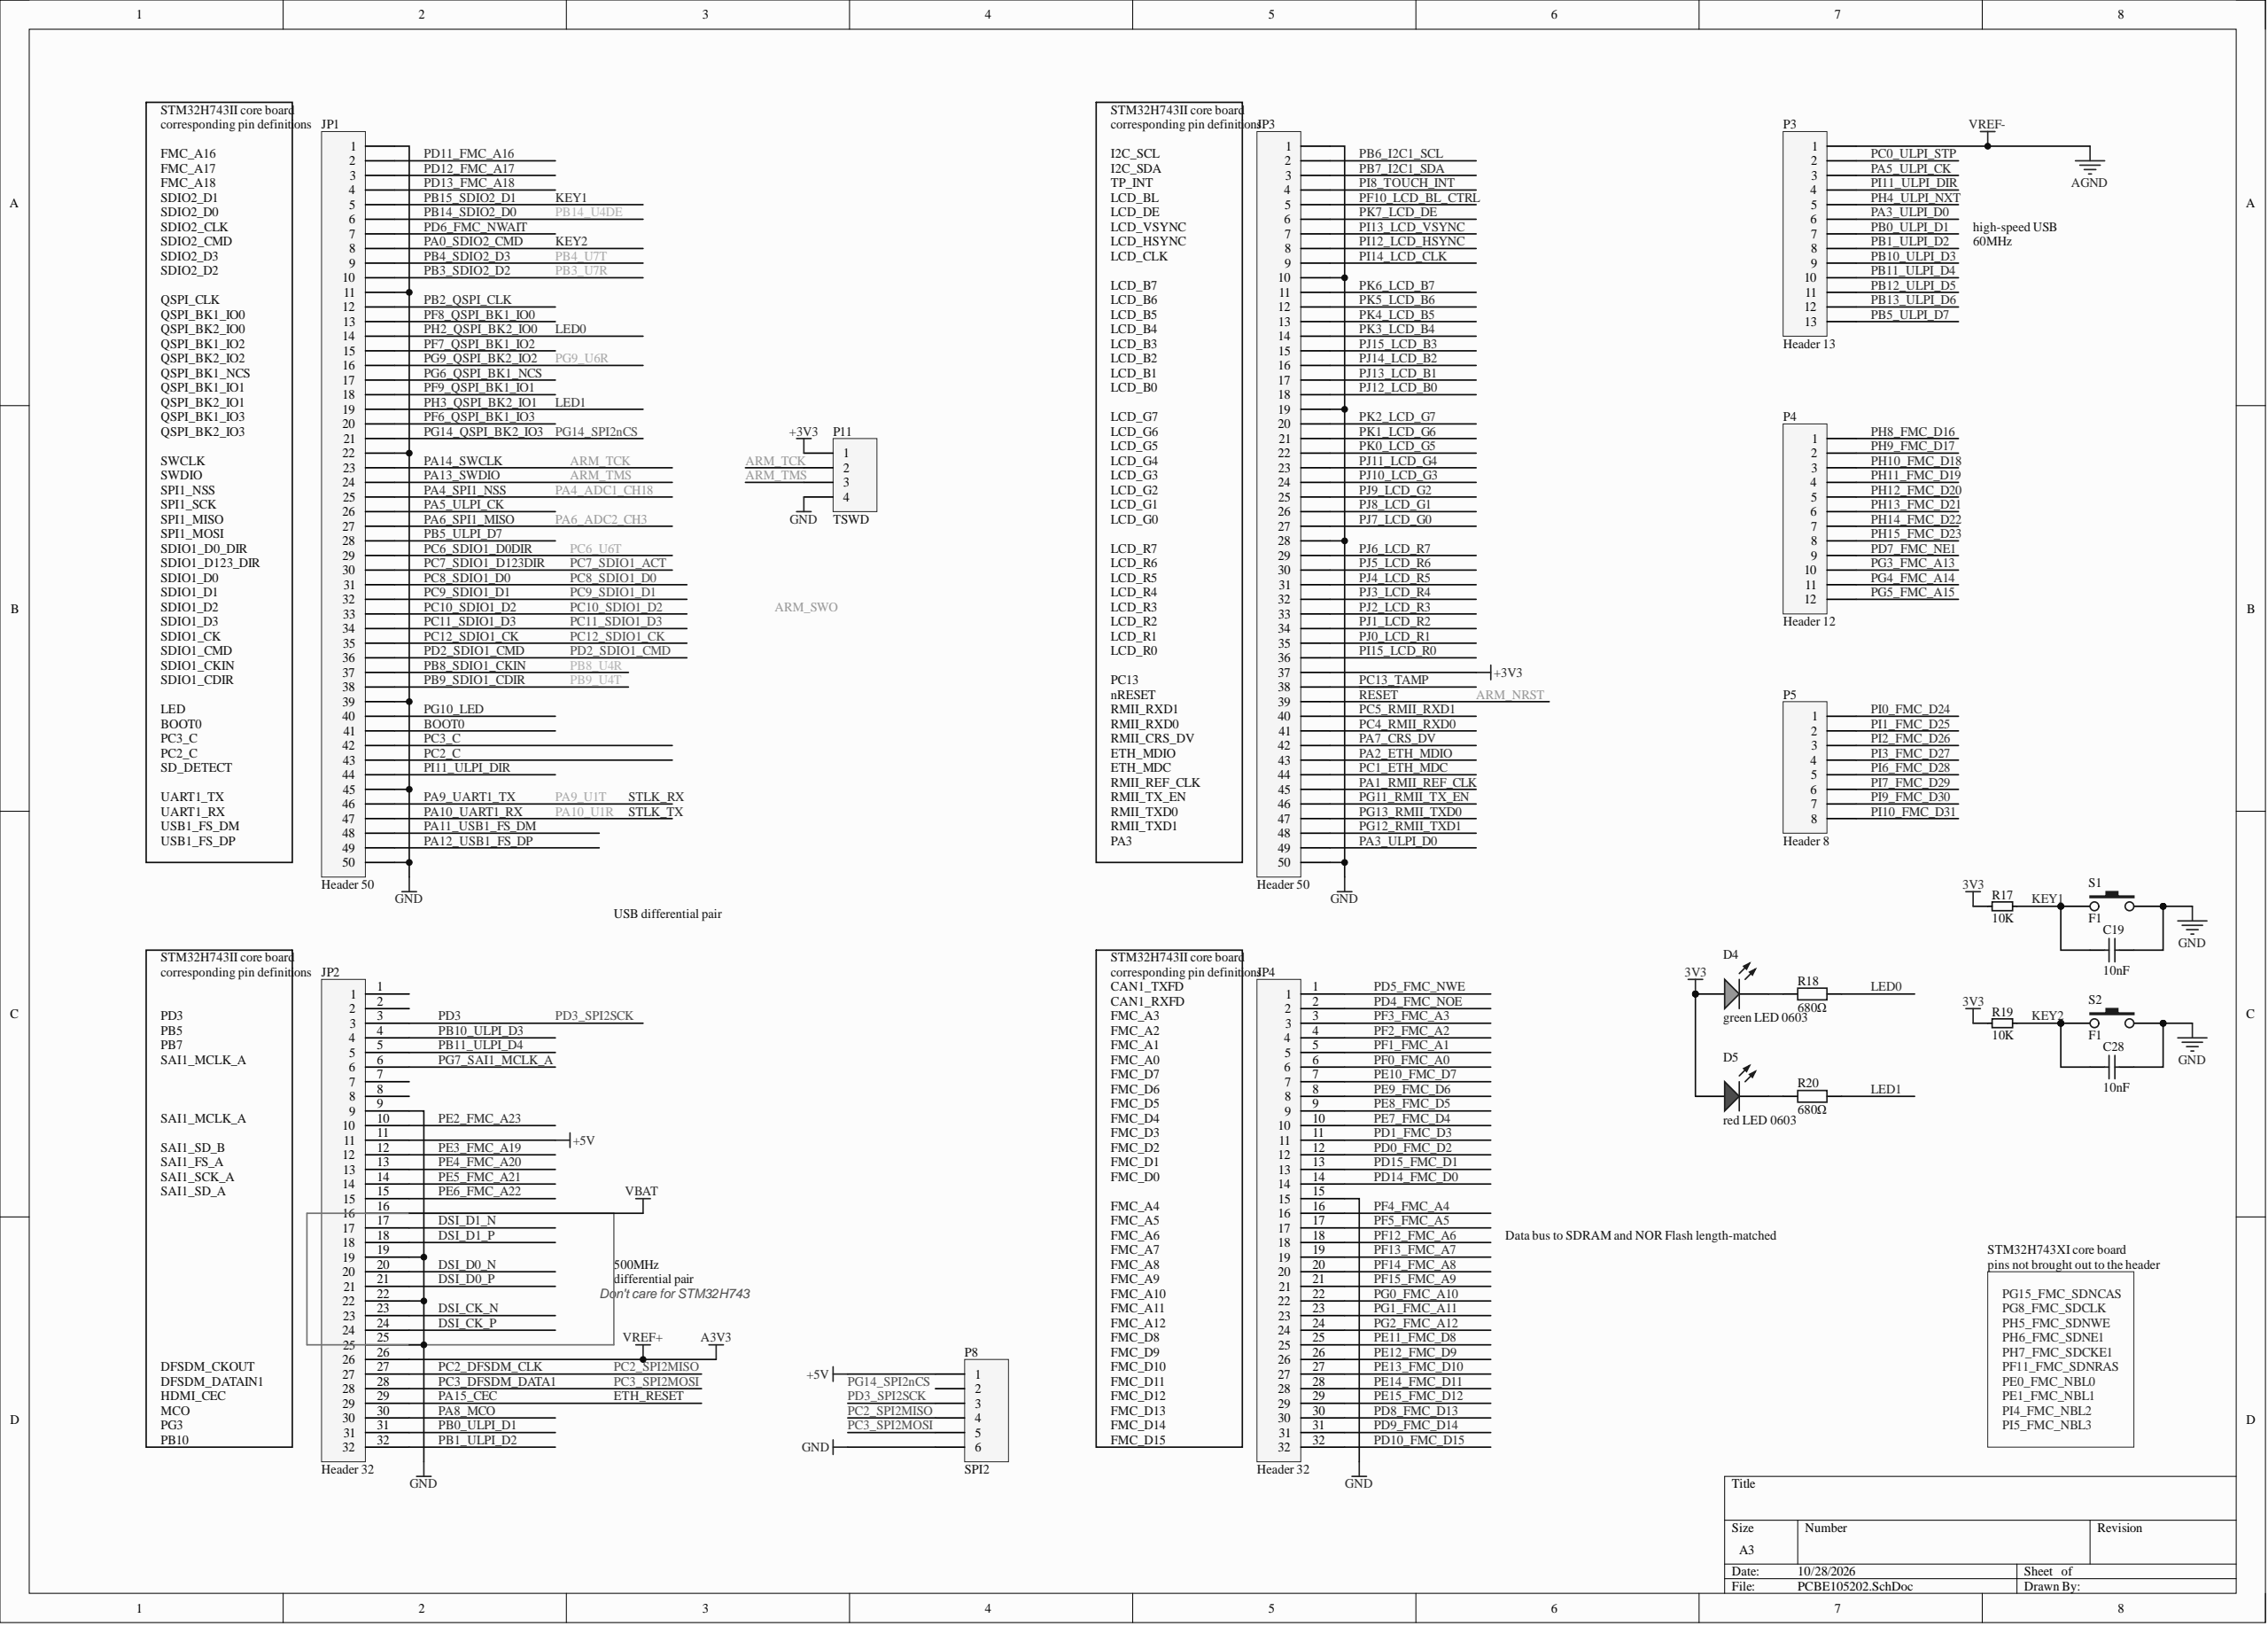Circuit board | Altium Designer | 181 parts | 141 nets | one sheet of the schematic
Parts on this sheet (reference | value | footprint):
C19 | 10nF | 0603_C
C28 | 10nF | 0603_C
JP1 | Header 50 | SIP-50-1.27-SMD-R
JP2 | Header 32 | SIP-32-1.27-SMD-R
JP3 | Header 50 | SIP-50-1.27-SMD
JP4 | Header 32 | SIP-32-1.27-SMD
P3 | Header 13 | CN13SM
P4 | Header 12 | CN12SM
P5 | Header 8 | CN8SM
P8 | SPI2 | HDR1X6
P11 | TSWD | HDR1X4
R17 | 10K | 0603_R
R18 | 680Ω | 0603_R
R19 | 10K | 0603_R
R20 | 680Ω | 0603_R
S1 | F1 | Reset_TE
S2 | F1 | Reset_TE
Nets of these parts (net: part-pin ...):
VBAT: JP2-16
PI11_ULPI_DIR: P3-4 JP1-44
PH4_ULPI_NXT: P3-5
PG13_RMII_TXD0: JP3-47
PG12_RMII_TXD1: JP3-48
PG11_RMII_TX_EN: JP3-46
PG9_QSPI_BK2_IO2: JP1-16
PD3: JP2-3 P8-3
PD2_SDIO1_CMD: JP1-36
PC12_SDIO1_CK: JP1-35
PC11_SDIO1_D3: JP1-34
PC10_SDIO1_D2: JP1-33
PC9_SDIO1_D1: JP1-32
PC8_SDIO1_D0: JP1-31
PC7_SDIO1_ACT: JP1-30
PC6_SDIO1_D0DIR: JP1-29
PC5_RMII_RXD1: JP3-40
PC4_RMII_RXD0: JP3-41
PC3_DFSDM_DATA1: JP2-28 P8-5
PC2_DFSDM_CLK: JP2-27 P8-4
PC1_ETH_MDC: JP3-44
PC0_ULPI_STP: P3-2
PB14_SDIO2_D0: JP1-6
PB13_ULPI_D6: P3-12
PB12_ULPI_D5: P3-11
PB11_ULPI_D4: JP2-5 P3-10
PB10_ULPI_D3: JP2-4 P3-9
PB9_SDIO1_CDIR: JP1-38
PB8_SDIO1_CKIN: JP1-37
PB5_ULPI_D7: P3-13 JP1-28
PB4_SDIO2_D3: JP1-9
PB3_SDIO2_D2: JP1-10
PB1_ULPI_D2: JP2-32 P3-8
PB0_ULPI_D1: JP2-31 P3-7
PA10_U1R: JP1-47
PA9_U1T: JP1-46
PA7_CRS_DV: JP3-42
PA6_ADC2_CH3: JP1-27
PA5_ULPI_CK: P3-3 JP1-26
PA4_ADC1_CH18: JP1-25
PA3_ULPI_D0: JP3-49 P3-6
PA2_ETH_MDIO: JP3-43
PA1_RMII_REF_CLK: JP3-45
NetD5_K: R20-1
NetD4_K: R18-1
LED1: R20-2 JP1-19
LED0: R18-2 JP1-14
KEY2: C28-1 R19-1 S2-1 JP1-8
KEY1: C19-1 R17-1 S1-1 JP1-5
GND: C19-2 C28-2 JP2-9 JP2-19 JP2-22 JP2-25 JP3-1 JP3-10 JP3-19 JP3-28 JP3-50 JP4-15 P8-6 P11-4 S1-2 S2-2 JP1-1 JP1-11 JP1-22 JP1-39 JP1-45 JP1-50
ETH_RESET: JP2-29
ARM_TMS: P11-3 JP1-24
ARM_TCK: P11-2 JP1-23
ARM_NRST: JP3-39
AGND: P3-1
A3V3: JP2-26
+5V: JP2-11 P8-1
+3V3: JP3-37 P11-1
3V3: R17-2 R19-2